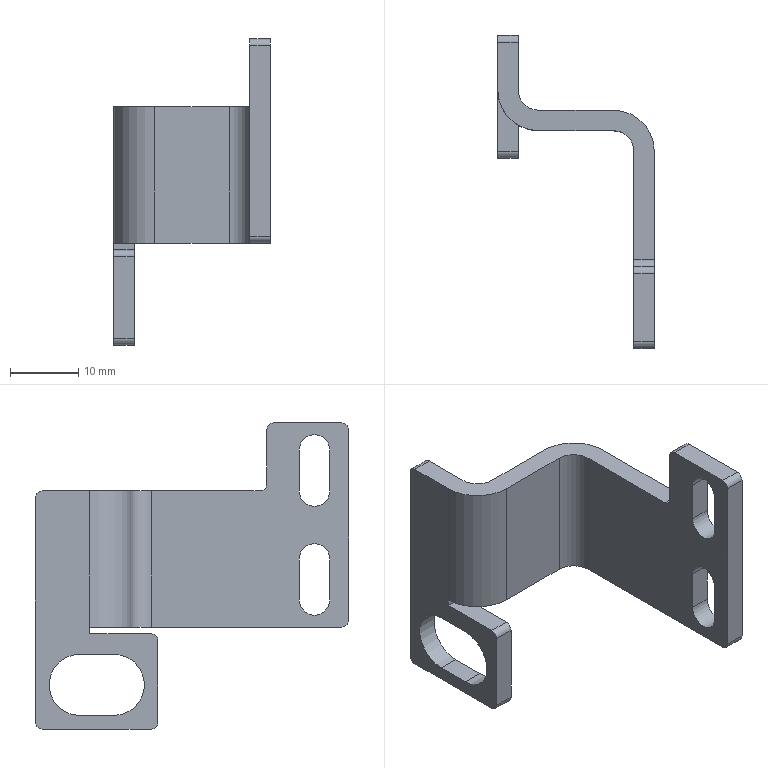Part | NX | features BREP 1 | 1 solid | 43 faces | box 23 x 46 x 45 mm | volume 4281 mm3 | plane 25 | cylinder 18 | commonest cylinder face diameters 2 x8 4.5 x4 6 x2 9 x2 12 x2
STEP:
#1=CARTESIAN_POINT('',(-6.,0.,5.));
#2=VERTEX_POINT('',#1);
#3=CARTESIAN_POINT('',(-17.,0.,5.));
#4=VERTEX_POINT('',#3);
#5=CARTESIAN_POINT('',(-20.,0.,5.));
#6=DIRECTION('',(-1.,0.,0.));
#7=VECTOR('',#6,1000.);
#8=LINE('',#5,#7);
#9=EDGE_CURVE('',#2,#4,#8,.T.);
#10=ORIENTED_EDGE('',*,*,#9,.F.);
#11=CARTESIAN_POINT('',(-6.,0.,-15.));
#12=VERTEX_POINT('',#11);
#13=CARTESIAN_POINT('',(-6.,0.,15.));
#14=DIRECTION('',(0.,0.,-1.));
#15=VECTOR('',#14,1000.);
#16=LINE('',#13,#15);
#17=EDGE_CURVE('',#2,#12,#16,.T.);
#18=ORIENTED_EDGE('',*,*,#17,.T.);
#19=CARTESIAN_POINT('',(-17.,0.,-15.));
#20=VERTEX_POINT('',#19);
#21=CARTESIAN_POINT('',(-20.,0.,-15.));
#22=DIRECTION('',(1.,0.,0.));
#23=VECTOR('',#22,1000.);
#24=LINE('',#21,#23);
#25=EDGE_CURVE('',#20,#12,#24,.T.);
#26=ORIENTED_EDGE('',*,*,#25,.F.);
#27=CARTESIAN_POINT('',(-17.,0.,15.));
#28=DIRECTION('',(0.,0.,-1.));
#29=VECTOR('',#28,1000.);
#30=LINE('',#27,#29);
#31=EDGE_CURVE('',#4,#20,#30,.T.);
#32=ORIENTED_EDGE('',*,*,#31,.F.);
#33=EDGE_LOOP('',(#10,#18,#26,#32));
#34=FACE_BOUND('',#33,.T.);
#35=CARTESIAN_POINT('',(-20.,0.,15.));
#36=DIRECTION('',(0.,1.,0.));
#37=DIRECTION('',(0.,0.,-1.));
#38=AXIS2_PLACEMENT_3D('',#35,#36,#37);
#39=PLANE('',#38);
#40=ADVANCED_FACE('',(#34),#39,.T.);
#41=CARTESIAN_POINT('',(-6.,-3.,5.));
#42=VERTEX_POINT('',#41);
#43=CARTESIAN_POINT('',(-6.,-3.,-15.));
#44=VERTEX_POINT('',#43);
#45=CARTESIAN_POINT('',(-6.,-3.,15.));
#46=DIRECTION('',(0.,0.,-1.));
#47=VECTOR('',#46,1000.);
#48=LINE('',#45,#47);
#49=EDGE_CURVE('',#42,#44,#48,.T.);
#50=ORIENTED_EDGE('',*,*,#49,.F.);
#51=CARTESIAN_POINT('',(-17.,-3.,5.));
#52=VERTEX_POINT('',#51);
#53=CARTESIAN_POINT('',(-20.,-3.,5.));
#54=DIRECTION('',(-1.,0.,0.));
#55=VECTOR('',#54,1000.);
#56=LINE('',#53,#55);
#57=EDGE_CURVE('',#42,#52,#56,.T.);
#58=ORIENTED_EDGE('',*,*,#57,.T.);
#59=CARTESIAN_POINT('',(-17.,-3.,-15.));
#60=VERTEX_POINT('',#59);
#61=CARTESIAN_POINT('',(-17.,-3.,15.));
#62=DIRECTION('',(0.,0.,-1.));
#63=VECTOR('',#62,1000.);
#64=LINE('',#61,#63);
#65=EDGE_CURVE('',#52,#60,#64,.T.);
#66=ORIENTED_EDGE('',*,*,#65,.T.);
#67=CARTESIAN_POINT('',(-20.,-3.,-15.));
#68=DIRECTION('',(1.,0.,0.));
#69=VECTOR('',#68,1000.);
#70=LINE('',#67,#69);
#71=EDGE_CURVE('',#60,#44,#70,.T.);
#72=ORIENTED_EDGE('',*,*,#71,.T.);
#73=EDGE_LOOP('',(#50,#58,#66,#72));
#74=FACE_BOUND('',#73,.T.);
#75=CARTESIAN_POINT('',(-20.,-3.,15.));
#76=DIRECTION('',(0.,1.,0.));
#77=DIRECTION('',(0.,0.,-1.));
#78=AXIS2_PLACEMENT_3D('',#75,#76,#77);
#79=PLANE('',#78);
#80=ADVANCED_FACE('',(#74),#79,.F.);
#81=CARTESIAN_POINT('',(0.,-24.,15.));
#82=VERTEX_POINT('',#81);
#83=CARTESIAN_POINT('',(0.,-34.,15.));
#84=VERTEX_POINT('',#83);
#85=CARTESIAN_POINT('',(0.,0.,15.));
#86=DIRECTION('',(0.,-1.,0.));
#87=VECTOR('',#86,1000.);
#88=LINE('',#85,#87);
#89=EDGE_CURVE('',#82,#84,#88,.T.);
#90=ORIENTED_EDGE('',*,*,#89,.F.);
#91=CARTESIAN_POINT('',(-3.,-24.,15.));
#92=VERTEX_POINT('',#91);
#93=CARTESIAN_POINT('',(-3.,-24.,15.));
#94=DIRECTION('',(-1.,0.,0.));
#95=VECTOR('',#94,1000.);
#96=LINE('',#93,#95);
#97=EDGE_CURVE('',#82,#92,#96,.T.);
#98=ORIENTED_EDGE('',*,*,#97,.T.);
#99=CARTESIAN_POINT('',(-3.,-34.,15.));
#100=VERTEX_POINT('',#99);
#101=CARTESIAN_POINT('',(-3.,0.,15.));
#102=DIRECTION('',(0.,-1.,0.));
#103=VECTOR('',#102,1000.);
#104=LINE('',#101,#103);
#105=EDGE_CURVE('',#92,#100,#104,.T.);
#106=ORIENTED_EDGE('',*,*,#105,.T.);
#107=CARTESIAN_POINT('',(-6.,-34.,15.));
#108=DIRECTION('',(1.,0.,0.));
#109=VECTOR('',#108,1000.);
#110=LINE('',#107,#109);
#111=EDGE_CURVE('',#100,#84,#110,.T.);
#112=ORIENTED_EDGE('',*,*,#111,.T.);
#113=EDGE_LOOP('',(#90,#98,#106,#112));
#114=FACE_BOUND('',#113,.T.);
#115=CARTESIAN_POINT('',(-6.,-3.,15.));
#116=DIRECTION('',(0.,0.,1.));
#117=DIRECTION('',(-1.,0.,0.));
#118=AXIS2_PLACEMENT_3D('',#115,#116,#117);
#119=PLANE('',#118);
#120=ADVANCED_FACE('',(#114),#119,.T.);
#121=CARTESIAN_POINT('',(-6.,0.,-15.));
#122=DIRECTION('',(0.,-1.,0.));
#123=VECTOR('',#122,1000.);
#124=LINE('',#121,#123);
#125=EDGE_CURVE('',#12,#44,#124,.T.);
#126=ORIENTED_EDGE('',*,*,#125,.F.);
#127=CARTESIAN_POINT('',(0.,-6.,-15.));
#128=VERTEX_POINT('',#127);
#129=CARTESIAN_POINT('',(-6.,-6.,-15.));
#130=DIRECTION('',(0.,0.,-1.));
#131=DIRECTION('',(1.,0.,0.));
#132=AXIS2_PLACEMENT_3D('',#129,#130,#131);
#133=CIRCLE('',#132,6.);
#134=EDGE_CURVE('',#12,#128,#133,.T.);
#135=ORIENTED_EDGE('',*,*,#134,.T.);
#136=CARTESIAN_POINT('',(-3.,-6.,-15.));
#137=VERTEX_POINT('',#136);
#138=CARTESIAN_POINT('',(-3.,-6.,-15.));
#139=DIRECTION('',(1.,0.,0.));
#140=VECTOR('',#139,1000.);
#141=LINE('',#138,#140);
#142=EDGE_CURVE('',#137,#128,#141,.T.);
#143=ORIENTED_EDGE('',*,*,#142,.F.);
#144=CARTESIAN_POINT('',(-6.,-6.,-15.));
#145=DIRECTION('',(0.,0.,-1.));
#146=DIRECTION('',(1.,0.,0.));
#147=AXIS2_PLACEMENT_3D('',#144,#145,#146);
#148=CIRCLE('',#147,3.);
#149=EDGE_CURVE('',#44,#137,#148,.T.);
#150=ORIENTED_EDGE('',*,*,#149,.F.);
#151=EDGE_LOOP('',(#126,#135,#143,#150));
#152=FACE_BOUND('',#151,.T.);
#153=CARTESIAN_POINT('',(-6.,0.,-15.));
#154=DIRECTION('',(0.,0.,-1.));
#155=DIRECTION('',(1.,0.,0.));
#156=AXIS2_PLACEMENT_3D('',#153,#154,#155);
#157=PLANE('',#156);
#158=ADVANCED_FACE('',(#152),#157,.T.);
#159=CARTESIAN_POINT('',(-17.,0.,-15.));
#160=DIRECTION('',(0.,-1.,0.));
#161=VECTOR('',#160,1000.);
#162=LINE('',#159,#161);
#163=EDGE_CURVE('',#20,#60,#162,.T.);
#164=ORIENTED_EDGE('',*,*,#163,.F.);
#165=ORIENTED_EDGE('',*,*,#25,.T.);
#166=ORIENTED_EDGE('',*,*,#125,.T.);
#167=ORIENTED_EDGE('',*,*,#71,.F.);
#168=EDGE_LOOP('',(#164,#165,#166,#167));
#169=FACE_BOUND('',#168,.T.);
#170=CARTESIAN_POINT('',(-3.,-6.,-15.));
#171=DIRECTION('',(0.,0.,-1.));
#172=DIRECTION('',(1.,0.,0.));
#173=AXIS2_PLACEMENT_3D('',#170,#171,#172);
#174=PLANE('',#173);
#175=ADVANCED_FACE('',(#169),#174,.T.);
#176=CARTESIAN_POINT('',(-3.,-27.75,11.));
#177=VERTEX_POINT('',#176);
#178=CARTESIAN_POINT('',(-3.,-27.75,5.));
#179=VERTEX_POINT('',#178);
#180=CARTESIAN_POINT('',(-3.,-27.75,11.));
#181=DIRECTION('',(0.,0.,-1.));
#182=VECTOR('',#181,1000.);
#183=LINE('',#180,#182);
#184=EDGE_CURVE('',#177,#179,#183,.T.);
#185=ORIENTED_EDGE('',*,*,#184,.F.);
#186=CARTESIAN_POINT('',(-3.,-32.25,11.));
#187=VERTEX_POINT('',#186);
#188=CARTESIAN_POINT('',(-3.,-30.,11.));
#189=DIRECTION('',(-1.,0.,0.));
#190=DIRECTION('',(0.,1.,0.));
#191=AXIS2_PLACEMENT_3D('',#188,#189,#190);
#192=CIRCLE('',#191,2.25);
#193=EDGE_CURVE('',#187,#177,#192,.T.);
#194=ORIENTED_EDGE('',*,*,#193,.F.);
#195=CARTESIAN_POINT('',(-3.,-32.25,5.));
#196=VERTEX_POINT('',#195);
#197=CARTESIAN_POINT('',(-3.,-32.25,11.));
#198=DIRECTION('',(0.,0.,1.));
#199=VECTOR('',#198,1000.);
#200=LINE('',#197,#199);
#201=EDGE_CURVE('',#196,#187,#200,.T.);
#202=ORIENTED_EDGE('',*,*,#201,.F.);
#203=CARTESIAN_POINT('',(-3.,-30.,5.));
#204=DIRECTION('',(-1.,0.,0.));
#205=DIRECTION('',(0.,1.,0.));
#206=AXIS2_PLACEMENT_3D('',#203,#204,#205);
#207=CIRCLE('',#206,2.25);
#208=EDGE_CURVE('',#179,#196,#207,.T.);
#209=ORIENTED_EDGE('',*,*,#208,.F.);
#210=EDGE_LOOP('',(#185,#194,#202,#209));
#211=FACE_BOUND('',#210,.T.);
#212=CARTESIAN_POINT('',(-3.,-27.75,-5.));
#213=VERTEX_POINT('',#212);
#214=CARTESIAN_POINT('',(-3.,-27.75,-11.));
#215=VERTEX_POINT('',#214);
#216=CARTESIAN_POINT('',(-3.,-27.75,-5.));
#217=DIRECTION('',(0.,0.,-1.));
#218=VECTOR('',#217,1000.);
#219=LINE('',#216,#218);
#220=EDGE_CURVE('',#213,#215,#219,.T.);
#221=ORIENTED_EDGE('',*,*,#220,.F.);
#222=CARTESIAN_POINT('',(-3.,-32.25,-5.));
#223=VERTEX_POINT('',#222);
#224=CARTESIAN_POINT('',(-3.,-30.,-5.));
#225=DIRECTION('',(-1.,0.,0.));
#226=DIRECTION('',(0.,1.,0.));
#227=AXIS2_PLACEMENT_3D('',#224,#225,#226);
#228=CIRCLE('',#227,2.25);
#229=EDGE_CURVE('',#223,#213,#228,.T.);
#230=ORIENTED_EDGE('',*,*,#229,.F.);
#231=CARTESIAN_POINT('',(-3.,-32.25,-11.));
#232=VERTEX_POINT('',#231);
#233=CARTESIAN_POINT('',(-3.,-32.25,-5.));
#234=DIRECTION('',(0.,0.,1.));
#235=VECTOR('',#234,1000.);
#236=LINE('',#233,#235);
#237=EDGE_CURVE('',#232,#223,#236,.T.);
#238=ORIENTED_EDGE('',*,*,#237,.F.);
#239=CARTESIAN_POINT('',(-3.,-30.,-11.));
#240=DIRECTION('',(-1.,0.,0.));
#241=DIRECTION('',(0.,1.,0.));
#242=AXIS2_PLACEMENT_3D('',#239,#240,#241);
#243=CIRCLE('',#242,2.25);
#244=EDGE_CURVE('',#215,#232,#243,.T.);
#245=ORIENTED_EDGE('',*,*,#244,.F.);
#246=EDGE_LOOP('',(#221,#230,#238,#245));
#247=FACE_BOUND('',#246,.T.);
#248=CARTESIAN_POINT('',(-3.,-34.,-15.));
#249=VERTEX_POINT('',#248);
#250=CARTESIAN_POINT('',(-3.,0.,-15.));
#251=DIRECTION('',(0.,-1.,0.));
#252=VECTOR('',#251,1000.);
#253=LINE('',#250,#252);
#254=EDGE_CURVE('',#137,#249,#253,.T.);
#255=ORIENTED_EDGE('',*,*,#254,.T.);
#256=CARTESIAN_POINT('',(-3.,-35.,-14.));
#257=VERTEX_POINT('',#256);
#258=CARTESIAN_POINT('',(-3.,-34.,-14.));
#259=DIRECTION('',(-1.,0.,0.));
#260=DIRECTION('',(0.,1.,0.));
#261=AXIS2_PLACEMENT_3D('',#258,#259,#260);
#262=CIRCLE('',#261,1.);
#263=EDGE_CURVE('',#249,#257,#262,.T.);
#264=ORIENTED_EDGE('',*,*,#263,.T.);
#265=CARTESIAN_POINT('',(-3.,-35.,14.));
#266=VERTEX_POINT('',#265);
#267=CARTESIAN_POINT('',(-3.,-35.,15.));
#268=DIRECTION('',(0.,0.,-1.));
#269=VECTOR('',#268,1000.);
#270=LINE('',#267,#269);
#271=EDGE_CURVE('',#266,#257,#270,.T.);
#272=ORIENTED_EDGE('',*,*,#271,.F.);
#273=CARTESIAN_POINT('',(-3.,-34.,14.));
#274=DIRECTION('',(-1.,0.,0.));
#275=DIRECTION('',(0.,1.,0.));
#276=AXIS2_PLACEMENT_3D('',#273,#274,#275);
#277=CIRCLE('',#276,1.);
#278=EDGE_CURVE('',#266,#100,#277,.T.);
#279=ORIENTED_EDGE('',*,*,#278,.T.);
#280=ORIENTED_EDGE('',*,*,#105,.F.);
#281=CARTESIAN_POINT('',(-3.,-23.,14.));
#282=VERTEX_POINT('',#281);
#283=CARTESIAN_POINT('',(-3.,-24.,14.));
#284=DIRECTION('',(-1.,0.,0.));
#285=DIRECTION('',(0.,1.,0.));
#286=AXIS2_PLACEMENT_3D('',#283,#284,#285);
#287=CIRCLE('',#286,1.);
#288=EDGE_CURVE('',#92,#282,#287,.T.);
#289=ORIENTED_EDGE('',*,*,#288,.T.);
#290=CARTESIAN_POINT('',(-3.,-23.,6.));
#291=VERTEX_POINT('',#290);
#292=CARTESIAN_POINT('',(-3.,-23.,15.));
#293=DIRECTION('',(0.,0.,-1.));
#294=VECTOR('',#293,1000.);
#295=LINE('',#292,#294);
#296=EDGE_CURVE('',#282,#291,#295,.T.);
#297=ORIENTED_EDGE('',*,*,#296,.T.);
#298=CARTESIAN_POINT('',(-3.,-22.,5.));
#299=VERTEX_POINT('',#298);
#300=CARTESIAN_POINT('',(-3.,-22.,6.));
#301=DIRECTION('',(1.,0.,0.));
#302=DIRECTION('',(0.,1.,0.));
#303=AXIS2_PLACEMENT_3D('',#300,#301,#302);
#304=CIRCLE('',#303,1.);
#305=EDGE_CURVE('',#291,#299,#304,.T.);
#306=ORIENTED_EDGE('',*,*,#305,.T.);
#307=CARTESIAN_POINT('',(-3.,-6.,5.));
#308=VERTEX_POINT('',#307);
#309=CARTESIAN_POINT('',(-3.,0.,5.));
#310=DIRECTION('',(0.,1.,0.));
#311=VECTOR('',#310,1000.);
#312=LINE('',#309,#311);
#313=EDGE_CURVE('',#299,#308,#312,.T.);
#314=ORIENTED_EDGE('',*,*,#313,.T.);
#315=CARTESIAN_POINT('',(-3.,-6.,15.));
#316=DIRECTION('',(0.,0.,-1.));
#317=VECTOR('',#316,1000.);
#318=LINE('',#315,#317);
#319=EDGE_CURVE('',#308,#137,#318,.T.);
#320=ORIENTED_EDGE('',*,*,#319,.T.);
#321=EDGE_LOOP('',(#255,#264,#272,#279,#280,#289,#297,#306,#314,#320));
#322=FACE_BOUND('',#321,.T.);
#323=CARTESIAN_POINT('',(-3.,0.,15.));
#324=DIRECTION('',(1.,0.,0.));
#325=DIRECTION('',(0.,-1.,0.));
#326=AXIS2_PLACEMENT_3D('',#323,#324,#325);
#327=PLANE('',#326);
#328=ADVANCED_FACE('',(#211,#247,#322),#327,.F.);
#329=ORIENTED_EDGE('',*,*,#271,.T.);
#330=CARTESIAN_POINT('',(0.,-35.,-14.));
#331=VERTEX_POINT('',#330);
#332=CARTESIAN_POINT('',(0.,-35.,-14.));
#333=DIRECTION('',(1.,0.,0.));
#334=VECTOR('',#333,1000.);
#335=LINE('',#332,#334);
#336=EDGE_CURVE('',#257,#331,#335,.T.);
#337=ORIENTED_EDGE('',*,*,#336,.T.);
#338=CARTESIAN_POINT('',(0.,-35.,14.));
#339=VERTEX_POINT('',#338);
#340=CARTESIAN_POINT('',(0.,-35.,15.));
#341=DIRECTION('',(0.,0.,-1.));
#342=VECTOR('',#341,1000.);
#343=LINE('',#340,#342);
#344=EDGE_CURVE('',#339,#331,#343,.T.);
#345=ORIENTED_EDGE('',*,*,#344,.F.);
#346=CARTESIAN_POINT('',(0.,-35.,14.));
#347=DIRECTION('',(-1.,0.,0.));
#348=VECTOR('',#347,1000.);
#349=LINE('',#346,#348);
#350=EDGE_CURVE('',#339,#266,#349,.T.);
#351=ORIENTED_EDGE('',*,*,#350,.T.);
#352=EDGE_LOOP('',(#329,#337,#345,#351));
#353=FACE_BOUND('',#352,.T.);
#354=CARTESIAN_POINT('',(0.,-35.,15.));
#355=DIRECTION('',(0.,-1.,0.));
#356=DIRECTION('',(0.,0.,1.));
#357=AXIS2_PLACEMENT_3D('',#354,#355,#356);
#358=PLANE('',#357);
#359=ADVANCED_FACE('',(#353),#358,.T.);
#360=ORIENTED_EDGE('',*,*,#344,.T.);
#361=CARTESIAN_POINT('',(0.,-34.,-15.));
#362=VERTEX_POINT('',#361);
#363=CARTESIAN_POINT('',(0.,-34.,-14.));
#364=DIRECTION('',(1.,0.,0.));
#365=DIRECTION('',(0.,1.,0.));
#366=AXIS2_PLACEMENT_3D('',#363,#364,#365);
#367=CIRCLE('',#366,1.);
#368=EDGE_CURVE('',#331,#362,#367,.T.);
#369=ORIENTED_EDGE('',*,*,#368,.T.);
#370=CARTESIAN_POINT('',(0.,0.,-15.));
#371=DIRECTION('',(0.,-1.,0.));
#372=VECTOR('',#371,1000.);
#373=LINE('',#370,#372);
#374=EDGE_CURVE('',#128,#362,#373,.T.);
#375=ORIENTED_EDGE('',*,*,#374,.F.);
#376=CARTESIAN_POINT('',(0.,-6.,5.));
#377=VERTEX_POINT('',#376);
#378=CARTESIAN_POINT('',(0.,-6.,15.));
#379=DIRECTION('',(0.,0.,-1.));
#380=VECTOR('',#379,1000.);
#381=LINE('',#378,#380);
#382=EDGE_CURVE('',#377,#128,#381,.T.);
#383=ORIENTED_EDGE('',*,*,#382,.F.);
#384=CARTESIAN_POINT('',(0.,-22.,5.));
#385=VERTEX_POINT('',#384);
#386=CARTESIAN_POINT('',(0.,11.,5.));
#387=DIRECTION('',(0.,1.,0.));
#388=VECTOR('',#387,1000.);
#389=LINE('',#386,#388);
#390=EDGE_CURVE('',#385,#377,#389,.T.);
#391=ORIENTED_EDGE('',*,*,#390,.F.);
#392=CARTESIAN_POINT('',(0.,-23.,6.));
#393=VERTEX_POINT('',#392);
#394=CARTESIAN_POINT('',(0.,-22.,6.));
#395=DIRECTION('',(-1.,0.,0.));
#396=DIRECTION('',(0.,1.,0.));
#397=AXIS2_PLACEMENT_3D('',#394,#395,#396);
#398=CIRCLE('',#397,1.);
#399=EDGE_CURVE('',#385,#393,#398,.T.);
#400=ORIENTED_EDGE('',*,*,#399,.T.);
#401=CARTESIAN_POINT('',(0.,-23.,14.));
#402=VERTEX_POINT('',#401);
#403=CARTESIAN_POINT('',(0.,-23.,5.));
#404=DIRECTION('',(0.,0.,-1.));
#405=VECTOR('',#404,1000.);
#406=LINE('',#403,#405);
#407=EDGE_CURVE('',#402,#393,#406,.T.);
#408=ORIENTED_EDGE('',*,*,#407,.F.);
#409=CARTESIAN_POINT('',(0.,-24.,14.));
#410=DIRECTION('',(1.,0.,0.));
#411=DIRECTION('',(0.,1.,0.));
#412=AXIS2_PLACEMENT_3D('',#409,#410,#411);
#413=CIRCLE('',#412,1.);
#414=EDGE_CURVE('',#402,#82,#413,.T.);
#415=ORIENTED_EDGE('',*,*,#414,.T.);
#416=ORIENTED_EDGE('',*,*,#89,.T.);
#417=CARTESIAN_POINT('',(0.,-34.,14.));
#418=DIRECTION('',(1.,0.,0.));
#419=DIRECTION('',(0.,1.,0.));
#420=AXIS2_PLACEMENT_3D('',#417,#418,#419);
#421=CIRCLE('',#420,1.);
#422=EDGE_CURVE('',#84,#339,#421,.T.);
#423=ORIENTED_EDGE('',*,*,#422,.T.);
#424=EDGE_LOOP('',(#360,#369,#375,#383,#391,#400,#408,#415,#416,#423));
#425=FACE_BOUND('',#424,.T.);
#426=CARTESIAN_POINT('',(0.,-27.75,11.));
#427=VERTEX_POINT('',#426);
#428=CARTESIAN_POINT('',(0.,-32.25,11.));
#429=VERTEX_POINT('',#428);
#430=CARTESIAN_POINT('',(0.,-30.,11.));
#431=DIRECTION('',(1.,0.,0.));
#432=DIRECTION('',(0.,1.,0.));
#433=AXIS2_PLACEMENT_3D('',#430,#431,#432);
#434=CIRCLE('',#433,2.25);
#435=EDGE_CURVE('',#427,#429,#434,.T.);
#436=ORIENTED_EDGE('',*,*,#435,.F.);
#437=CARTESIAN_POINT('',(0.,-27.75,5.));
#438=VERTEX_POINT('',#437);
#439=CARTESIAN_POINT('',(0.,-27.75,11.));
#440=DIRECTION('',(0.,0.,1.));
#441=VECTOR('',#440,1000.);
#442=LINE('',#439,#441);
#443=EDGE_CURVE('',#438,#427,#442,.T.);
#444=ORIENTED_EDGE('',*,*,#443,.F.);
#445=CARTESIAN_POINT('',(0.,-32.25,5.));
#446=VERTEX_POINT('',#445);
#447=CARTESIAN_POINT('',(0.,-30.,5.));
#448=DIRECTION('',(1.,0.,0.));
#449=DIRECTION('',(0.,1.,0.));
#450=AXIS2_PLACEMENT_3D('',#447,#448,#449);
#451=CIRCLE('',#450,2.25);
#452=EDGE_CURVE('',#446,#438,#451,.T.);
#453=ORIENTED_EDGE('',*,*,#452,.F.);
#454=CARTESIAN_POINT('',(0.,-32.25,11.));
#455=DIRECTION('',(0.,0.,-1.));
#456=VECTOR('',#455,1000.);
#457=LINE('',#454,#456);
#458=EDGE_CURVE('',#429,#446,#457,.T.);
#459=ORIENTED_EDGE('',*,*,#458,.F.);
#460=EDGE_LOOP('',(#436,#444,#453,#459));
#461=FACE_BOUND('',#460,.T.);
#462=CARTESIAN_POINT('',(0.,-27.75,-5.));
#463=VERTEX_POINT('',#462);
#464=CARTESIAN_POINT('',(0.,-32.25,-5.));
#465=VERTEX_POINT('',#464);
#466=CARTESIAN_POINT('',(0.,-30.,-5.));
#467=DIRECTION('',(1.,0.,0.));
#468=DIRECTION('',(0.,1.,0.));
#469=AXIS2_PLACEMENT_3D('',#466,#467,#468);
#470=CIRCLE('',#469,2.25);
#471=EDGE_CURVE('',#463,#465,#470,.T.);
#472=ORIENTED_EDGE('',*,*,#471,.F.);
#473=CARTESIAN_POINT('',(0.,-27.75,-11.));
#474=VERTEX_POINT('',#473);
#475=CARTESIAN_POINT('',(0.,-27.75,-5.));
#476=DIRECTION('',(0.,0.,1.));
#477=VECTOR('',#476,1000.);
#478=LINE('',#475,#477);
#479=EDGE_CURVE('',#474,#463,#478,.T.);
#480=ORIENTED_EDGE('',*,*,#479,.F.);
#481=CARTESIAN_POINT('',(0.,-32.25,-11.));
#482=VERTEX_POINT('',#481);
#483=CARTESIAN_POINT('',(0.,-30.,-11.));
#484=DIRECTION('',(1.,0.,0.));
#485=DIRECTION('',(0.,1.,0.));
#486=AXIS2_PLACEMENT_3D('',#483,#484,#485);
#487=CIRCLE('',#486,2.25);
#488=EDGE_CURVE('',#482,#474,#487,.T.);
#489=ORIENTED_EDGE('',*,*,#488,.F.);
#490=CARTESIAN_POINT('',(0.,-32.25,-5.));
#491=DIRECTION('',(0.,0.,-1.));
#492=VECTOR('',#491,1000.);
#493=LINE('',#490,#492);
#494=EDGE_CURVE('',#465,#482,#493,.T.);
#495=ORIENTED_EDGE('',*,*,#494,.F.);
#496=EDGE_LOOP('',(#472,#480,#489,#495));
#497=FACE_BOUND('',#496,.T.);
#498=CARTESIAN_POINT('',(0.,0.,15.));
#499=DIRECTION('',(1.,0.,0.));
#500=DIRECTION('',(0.,-1.,0.));
#501=AXIS2_PLACEMENT_3D('',#498,#499,#500);
#502=PLANE('',#501);
#503=ADVANCED_FACE('',(#425,#461,#497),#502,.T.);
#504=CARTESIAN_POINT('',(-6.,-6.,5.));
#505=DIRECTION('',(0.,0.,1.));
#506=DIRECTION('',(0.,1.,0.));
#507=AXIS2_PLACEMENT_3D('',#504,#505,#506);
#508=CIRCLE('',#507,6.);
#509=EDGE_CURVE('',#377,#2,#508,.T.);
#510=ORIENTED_EDGE('',*,*,#509,.F.);
#511=ORIENTED_EDGE('',*,*,#382,.T.);
#512=ORIENTED_EDGE('',*,*,#134,.F.);
#513=ORIENTED_EDGE('',*,*,#17,.F.);
#514=EDGE_LOOP('',(#510,#511,#512,#513));
#515=FACE_BOUND('',#514,.T.);
#516=CARTESIAN_POINT('',(-6.,-6.,15.));
#517=DIRECTION('',(0.,0.,-1.));
#518=DIRECTION('',(1.,0.,0.));
#519=AXIS2_PLACEMENT_3D('',#516,#517,#518);
#520=CYLINDRICAL_SURFACE('',#519,6.);
#521=ADVANCED_FACE('',(#515),#520,.T.);
#522=ORIENTED_EDGE('',*,*,#319,.F.);
#523=CARTESIAN_POINT('',(-6.,-6.,5.));
#524=DIRECTION('',(0.,0.,1.));
#525=DIRECTION('',(0.,1.,0.));
#526=AXIS2_PLACEMENT_3D('',#523,#524,#525);
#527=CIRCLE('',#526,3.);
#528=EDGE_CURVE('',#308,#42,#527,.T.);
#529=ORIENTED_EDGE('',*,*,#528,.T.);
#530=ORIENTED_EDGE('',*,*,#49,.T.);
#531=ORIENTED_EDGE('',*,*,#149,.T.);
#532=EDGE_LOOP('',(#522,#529,#530,#531));
#533=FACE_BOUND('',#532,.T.);
#534=CARTESIAN_POINT('',(-6.,-6.,15.));
#535=DIRECTION('',(0.,0.,-1.));
#536=DIRECTION('',(1.,0.,0.));
#537=AXIS2_PLACEMENT_3D('',#534,#535,#536);
#538=CYLINDRICAL_SURFACE('',#537,3.);
#539=ADVANCED_FACE('',(#533),#538,.F.);
#540=ORIENTED_EDGE('',*,*,#374,.T.);
#541=CARTESIAN_POINT('',(-3.,-34.,-15.));
#542=DIRECTION('',(-1.,0.,0.));
#543=VECTOR('',#542,1000.);
#544=LINE('',#541,#543);
#545=EDGE_CURVE('',#362,#249,#544,.T.);
#546=ORIENTED_EDGE('',*,*,#545,.T.);
#547=ORIENTED_EDGE('',*,*,#254,.F.);
#548=ORIENTED_EDGE('',*,*,#142,.T.);
#549=EDGE_LOOP('',(#540,#546,#547,#548));
#550=FACE_BOUND('',#549,.T.);
#551=CARTESIAN_POINT('',(-6.,-6.,-15.));
#552=DIRECTION('',(0.,0.,1.));
#553=DIRECTION('',(-1.,0.,0.));
#554=AXIS2_PLACEMENT_3D('',#551,#552,#553);
#555=PLANE('',#554);
#556=ADVANCED_FACE('',(#550),#555,.F.);
#557=CARTESIAN_POINT('',(-20.,3.,-15.));
#558=VERTEX_POINT('',#557);
#559=CARTESIAN_POINT('',(-23.,3.,-15.));
#560=VERTEX_POINT('',#559);
#561=CARTESIAN_POINT('',(-20.,3.,-15.));
#562=DIRECTION('',(-1.,0.,0.));
#563=VECTOR('',#562,1000.);
#564=LINE('',#561,#563);
#565=EDGE_CURVE('',#558,#560,#564,.T.);
#566=ORIENTED_EDGE('',*,*,#565,.F.);
#567=CARTESIAN_POINT('',(-17.,3.,-15.));
#568=DIRECTION('',(0.,0.,-1.));
#569=DIRECTION('',(1.,0.,0.));
#570=AXIS2_PLACEMENT_3D('',#567,#568,#569);
#571=CIRCLE('',#570,3.);
#572=EDGE_CURVE('',#20,#558,#571,.T.);
#573=ORIENTED_EDGE('',*,*,#572,.F.);
#574=ORIENTED_EDGE('',*,*,#163,.T.);
#575=CARTESIAN_POINT('',(-17.,3.,-15.));
#576=DIRECTION('',(0.,0.,-1.));
#577=DIRECTION('',(1.,0.,0.));
#578=AXIS2_PLACEMENT_3D('',#575,#576,#577);
#579=CIRCLE('',#578,6.);
#580=EDGE_CURVE('',#60,#560,#579,.T.);
#581=ORIENTED_EDGE('',*,*,#580,.T.);
#582=EDGE_LOOP('',(#566,#573,#574,#581));
#583=FACE_BOUND('',#582,.T.);
#584=CARTESIAN_POINT('',(-17.,3.,-15.));
#585=DIRECTION('',(0.,0.,-1.));
#586=DIRECTION('',(1.,0.,0.));
#587=AXIS2_PLACEMENT_3D('',#584,#585,#586);
#588=PLANE('',#587);
#589=ADVANCED_FACE('',(#583),#588,.T.);
#590=CARTESIAN_POINT('',(-23.,3.,5.));
#591=VERTEX_POINT('',#590);
#592=CARTESIAN_POINT('',(-17.,3.,5.));
#593=DIRECTION('',(0.,0.,1.));
#594=DIRECTION('',(0.,1.,0.));
#595=AXIS2_PLACEMENT_3D('',#592,#593,#594);
#596=CIRCLE('',#595,6.);
#597=EDGE_CURVE('',#591,#52,#596,.T.);
#598=ORIENTED_EDGE('',*,*,#597,.F.);
#599=CARTESIAN_POINT('',(-23.,3.,0.));
#600=DIRECTION('',(0.,0.,-1.));
#601=VECTOR('',#600,1000.);
#602=LINE('',#599,#601);
#603=EDGE_CURVE('',#591,#560,#602,.T.);
#604=ORIENTED_EDGE('',*,*,#603,.T.);
#605=ORIENTED_EDGE('',*,*,#580,.F.);
#606=ORIENTED_EDGE('',*,*,#65,.F.);
#607=EDGE_LOOP('',(#598,#604,#605,#606));
#608=FACE_BOUND('',#607,.T.);
#609=CARTESIAN_POINT('',(-17.,3.,15.));
#610=DIRECTION('',(0.,0.,1.));
#611=DIRECTION('',(1.,0.,0.));
#612=AXIS2_PLACEMENT_3D('',#609,#610,#611);
#613=CYLINDRICAL_SURFACE('',#612,6.);
#614=ADVANCED_FACE('',(#608),#613,.T.);
#615=CARTESIAN_POINT('',(-20.,3.,5.));
#616=VERTEX_POINT('',#615);
#617=CARTESIAN_POINT('',(-20.,3.,-15.));
#618=DIRECTION('',(0.,0.,1.));
#619=VECTOR('',#618,1000.);
#620=LINE('',#617,#619);
#621=EDGE_CURVE('',#558,#616,#620,.T.);
#622=ORIENTED_EDGE('',*,*,#621,.T.);
#623=CARTESIAN_POINT('',(-17.,3.,5.));
#624=DIRECTION('',(0.,0.,1.));
#625=DIRECTION('',(0.,1.,0.));
#626=AXIS2_PLACEMENT_3D('',#623,#624,#625);
#627=CIRCLE('',#626,3.);
#628=EDGE_CURVE('',#616,#4,#627,.T.);
#629=ORIENTED_EDGE('',*,*,#628,.T.);
#630=ORIENTED_EDGE('',*,*,#31,.T.);
#631=ORIENTED_EDGE('',*,*,#572,.T.);
#632=EDGE_LOOP('',(#622,#629,#630,#631));
#633=FACE_BOUND('',#632,.T.);
#634=CARTESIAN_POINT('',(-17.,3.,15.));
#635=DIRECTION('',(0.,0.,1.));
#636=DIRECTION('',(1.,0.,0.));
#637=AXIS2_PLACEMENT_3D('',#634,#635,#636);
#638=CYLINDRICAL_SURFACE('',#637,3.);
#639=ADVANCED_FACE('',(#633),#638,.F.);
#640=CARTESIAN_POINT('',(-23.,4.5,-28.));
#641=VERTEX_POINT('',#640);
#642=CARTESIAN_POINT('',(-23.,-0.5,-28.));
#643=VERTEX_POINT('',#642);
#644=CARTESIAN_POINT('',(-23.,4.5,-28.));
#645=DIRECTION('',(0.,-1.,0.));
#646=VECTOR('',#645,1000.);
#647=LINE('',#644,#646);
#648=EDGE_CURVE('',#641,#643,#647,.T.);
#649=ORIENTED_EDGE('',*,*,#648,.F.);
#650=CARTESIAN_POINT('',(-23.,4.5,-19.));
#651=VERTEX_POINT('',#650);
#652=CARTESIAN_POINT('',(-23.,4.5,-23.5));
#653=DIRECTION('',(-1.,0.,0.));
#654=DIRECTION('',(0.,1.,0.));
#655=AXIS2_PLACEMENT_3D('',#652,#653,#654);
#656=CIRCLE('',#655,4.5);
#657=EDGE_CURVE('',#651,#641,#656,.T.);
#658=ORIENTED_EDGE('',*,*,#657,.F.);
#659=CARTESIAN_POINT('',(-23.,-0.5,-19.));
#660=VERTEX_POINT('',#659);
#661=CARTESIAN_POINT('',(-23.,4.5,-19.));
#662=DIRECTION('',(0.,1.,0.));
#663=VECTOR('',#662,1000.);
#664=LINE('',#661,#663);
#665=EDGE_CURVE('',#660,#651,#664,.T.);
#666=ORIENTED_EDGE('',*,*,#665,.F.);
#667=CARTESIAN_POINT('',(-23.,-0.5,-23.5));
#668=DIRECTION('',(-1.,0.,0.));
#669=DIRECTION('',(0.,1.,0.));
#670=AXIS2_PLACEMENT_3D('',#667,#668,#669);
#671=CIRCLE('',#670,4.5);
#672=EDGE_CURVE('',#643,#660,#671,.T.);
#673=ORIENTED_EDGE('',*,*,#672,.F.);
#674=EDGE_LOOP('',(#649,#658,#666,#673));
#675=FACE_BOUND('',#674,.T.);
#676=CARTESIAN_POINT('',(-23.,11.,4.));
#677=VERTEX_POINT('',#676);
#678=CARTESIAN_POINT('',(-23.,11.,-29.));
#679=VERTEX_POINT('',#678);
#680=CARTESIAN_POINT('',(-23.,11.,-15.));
#681=DIRECTION('',(0.,0.,-1.));
#682=VECTOR('',#681,1000.);
#683=LINE('',#680,#682);
#684=EDGE_CURVE('',#677,#679,#683,.T.);
#685=ORIENTED_EDGE('',*,*,#684,.T.);
#686=CARTESIAN_POINT('',(-23.,10.,-30.));
#687=VERTEX_POINT('',#686);
#688=CARTESIAN_POINT('',(-23.,10.,-29.));
#689=DIRECTION('',(-1.,0.,0.));
#690=DIRECTION('',(0.,1.,0.));
#691=AXIS2_PLACEMENT_3D('',#688,#689,#690);
#692=CIRCLE('',#691,1.);
#693=EDGE_CURVE('',#679,#687,#692,.T.);
#694=ORIENTED_EDGE('',*,*,#693,.T.);
#695=CARTESIAN_POINT('',(-23.,-6.,-30.));
#696=VERTEX_POINT('',#695);
#697=CARTESIAN_POINT('',(-23.,11.,-30.));
#698=DIRECTION('',(0.,-1.,0.));
#699=VECTOR('',#698,1000.);
#700=LINE('',#697,#699);
#701=EDGE_CURVE('',#687,#696,#700,.T.);
#702=ORIENTED_EDGE('',*,*,#701,.T.);
#703=CARTESIAN_POINT('',(-23.,-7.,-29.));
#704=VERTEX_POINT('',#703);
#705=CARTESIAN_POINT('',(-23.,-6.,-29.));
#706=DIRECTION('',(-1.,0.,0.));
#707=DIRECTION('',(0.,1.,0.));
#708=AXIS2_PLACEMENT_3D('',#705,#706,#707);
#709=CIRCLE('',#708,1.);
#710=EDGE_CURVE('',#696,#704,#709,.T.);
#711=ORIENTED_EDGE('',*,*,#710,.T.);
#712=CARTESIAN_POINT('',(-23.,-7.,-17.));
#713=VERTEX_POINT('',#712);
#714=CARTESIAN_POINT('',(-23.,-7.,-30.));
#715=DIRECTION('',(0.,0.,1.));
#716=VECTOR('',#715,1000.);
#717=LINE('',#714,#716);
#718=EDGE_CURVE('',#704,#713,#717,.T.);
#719=ORIENTED_EDGE('',*,*,#718,.T.);
#720=CARTESIAN_POINT('',(-23.,-6.,-16.));
#721=VERTEX_POINT('',#720);
#722=CARTESIAN_POINT('',(-23.,-6.,-17.));
#723=DIRECTION('',(-1.,0.,0.));
#724=DIRECTION('',(0.,1.,0.));
#725=AXIS2_PLACEMENT_3D('',#722,#723,#724);
#726=CIRCLE('',#725,1.);
#727=EDGE_CURVE('',#713,#721,#726,.T.);
#728=ORIENTED_EDGE('',*,*,#727,.T.);
#729=CARTESIAN_POINT('',(-23.,3.,-16.));
#730=VERTEX_POINT('',#729);
#731=CARTESIAN_POINT('',(-23.,-7.,-16.));
#732=DIRECTION('',(0.,1.,0.));
#733=VECTOR('',#732,1000.);
#734=LINE('',#731,#733);
#735=EDGE_CURVE('',#721,#730,#734,.T.);
#736=ORIENTED_EDGE('',*,*,#735,.T.);
#737=CARTESIAN_POINT('',(-23.,3.,-16.));
#738=DIRECTION('',(0.,0.,1.));
#739=VECTOR('',#738,1000.);
#740=LINE('',#737,#739);
#741=EDGE_CURVE('',#730,#560,#740,.T.);
#742=ORIENTED_EDGE('',*,*,#741,.T.);
#743=ORIENTED_EDGE('',*,*,#603,.F.);
#744=CARTESIAN_POINT('',(-23.,10.,5.));
#745=VERTEX_POINT('',#744);
#746=CARTESIAN_POINT('',(-23.,11.,5.));
#747=DIRECTION('',(0.,-1.,0.));
#748=VECTOR('',#747,1000.);
#749=LINE('',#746,#748);
#750=EDGE_CURVE('',#745,#591,#749,.T.);
#751=ORIENTED_EDGE('',*,*,#750,.F.);
#752=CARTESIAN_POINT('',(-23.,10.,4.));
#753=DIRECTION('',(-1.,0.,0.));
#754=DIRECTION('',(0.,1.,0.));
#755=AXIS2_PLACEMENT_3D('',#752,#753,#754);
#756=CIRCLE('',#755,1.);
#757=EDGE_CURVE('',#745,#677,#756,.T.);
#758=ORIENTED_EDGE('',*,*,#757,.T.);
#759=EDGE_LOOP('',(#685,#694,#702,#711,#719,#728,#736,#742,#743,#751,#758));
#760=FACE_BOUND('',#759,.T.);
#761=CARTESIAN_POINT('',(-23.,0.,0.));
#762=DIRECTION('',(1.,0.,0.));
#763=DIRECTION('',(0.,-1.,0.));
#764=AXIS2_PLACEMENT_3D('',#761,#762,#763);
#765=PLANE('',#764);
#766=ADVANCED_FACE('',(#675,#760),#765,.F.);
#767=CARTESIAN_POINT('',(-20.,4.5,-28.));
#768=VERTEX_POINT('',#767);
#769=CARTESIAN_POINT('',(-20.,4.5,-19.));
#770=VERTEX_POINT('',#769);
#771=CARTESIAN_POINT('',(-20.,4.5,-23.5));
#772=DIRECTION('',(1.,0.,0.));
#773=DIRECTION('',(0.,1.,0.));
#774=AXIS2_PLACEMENT_3D('',#771,#772,#773);
#775=CIRCLE('',#774,4.5);
#776=EDGE_CURVE('',#768,#770,#775,.T.);
#777=ORIENTED_EDGE('',*,*,#776,.F.);
#778=CARTESIAN_POINT('',(-20.,-0.5,-28.));
#779=VERTEX_POINT('',#778);
#780=CARTESIAN_POINT('',(-20.,4.5,-28.));
#781=DIRECTION('',(0.,1.,0.));
#782=VECTOR('',#781,1000.);
#783=LINE('',#780,#782);
#784=EDGE_CURVE('',#779,#768,#783,.T.);
#785=ORIENTED_EDGE('',*,*,#784,.F.);
#786=CARTESIAN_POINT('',(-20.,-0.5,-19.));
#787=VERTEX_POINT('',#786);
#788=CARTESIAN_POINT('',(-20.,-0.5,-23.5));
#789=DIRECTION('',(1.,0.,0.));
#790=DIRECTION('',(0.,1.,0.));
#791=AXIS2_PLACEMENT_3D('',#788,#789,#790);
#792=CIRCLE('',#791,4.5);
#793=EDGE_CURVE('',#787,#779,#792,.T.);
#794=ORIENTED_EDGE('',*,*,#793,.F.);
#795=CARTESIAN_POINT('',(-20.,4.5,-19.));
#796=DIRECTION('',(0.,-1.,0.));
#797=VECTOR('',#796,1000.);
#798=LINE('',#795,#797);
#799=EDGE_CURVE('',#770,#787,#798,.T.);
#800=ORIENTED_EDGE('',*,*,#799,.F.);
#801=EDGE_LOOP('',(#777,#785,#794,#800));
#802=FACE_BOUND('',#801,.T.);
#803=CARTESIAN_POINT('',(-20.,10.,-30.));
#804=VERTEX_POINT('',#803);
#805=CARTESIAN_POINT('',(-20.,-6.,-30.));
#806=VERTEX_POINT('',#805);
#807=CARTESIAN_POINT('',(-20.,11.,-30.));
#808=DIRECTION('',(0.,-1.,0.));
#809=VECTOR('',#808,1000.);
#810=LINE('',#807,#809);
#811=EDGE_CURVE('',#804,#806,#810,.T.);
#812=ORIENTED_EDGE('',*,*,#811,.F.);
#813=CARTESIAN_POINT('',(-20.,11.,-29.));
#814=VERTEX_POINT('',#813);
#815=CARTESIAN_POINT('',(-20.,10.,-29.));
#816=DIRECTION('',(1.,0.,0.));
#817=DIRECTION('',(0.,1.,0.));
#818=AXIS2_PLACEMENT_3D('',#815,#816,#817);
#819=CIRCLE('',#818,1.);
#820=EDGE_CURVE('',#804,#814,#819,.T.);
#821=ORIENTED_EDGE('',*,*,#820,.T.);
#822=CARTESIAN_POINT('',(-20.,11.,4.));
#823=VERTEX_POINT('',#822);
#824=CARTESIAN_POINT('',(-20.,11.,-15.));
#825=DIRECTION('',(0.,0.,-1.));
#826=VECTOR('',#825,1000.);
#827=LINE('',#824,#826);
#828=EDGE_CURVE('',#823,#814,#827,.T.);
#829=ORIENTED_EDGE('',*,*,#828,.F.);
#830=CARTESIAN_POINT('',(-20.,10.,5.));
#831=VERTEX_POINT('',#830);
#832=CARTESIAN_POINT('',(-20.,10.,4.));
#833=DIRECTION('',(1.,0.,0.));
#834=DIRECTION('',(0.,1.,0.));
#835=AXIS2_PLACEMENT_3D('',#832,#833,#834);
#836=CIRCLE('',#835,1.);
#837=EDGE_CURVE('',#823,#831,#836,.T.);
#838=ORIENTED_EDGE('',*,*,#837,.T.);
#839=CARTESIAN_POINT('',(-20.,0.,5.));
#840=DIRECTION('',(0.,1.,0.));
#841=VECTOR('',#840,1000.);
#842=LINE('',#839,#841);
#843=EDGE_CURVE('',#616,#831,#842,.T.);
#844=ORIENTED_EDGE('',*,*,#843,.F.);
#845=ORIENTED_EDGE('',*,*,#621,.F.);
#846=CARTESIAN_POINT('',(-20.,3.,-16.));
#847=VERTEX_POINT('',#846);
#848=CARTESIAN_POINT('',(-20.,3.,-16.));
#849=DIRECTION('',(0.,0.,1.));
#850=VECTOR('',#849,1000.);
#851=LINE('',#848,#850);
#852=EDGE_CURVE('',#847,#558,#851,.T.);
#853=ORIENTED_EDGE('',*,*,#852,.F.);
#854=CARTESIAN_POINT('',(-20.,-6.,-16.));
#855=VERTEX_POINT('',#854);
#856=CARTESIAN_POINT('',(-20.,-7.,-16.));
#857=DIRECTION('',(0.,1.,0.));
#858=VECTOR('',#857,1000.);
#859=LINE('',#856,#858);
#860=EDGE_CURVE('',#855,#847,#859,.T.);
#861=ORIENTED_EDGE('',*,*,#860,.F.);
#862=CARTESIAN_POINT('',(-20.,-7.,-17.));
#863=VERTEX_POINT('',#862);
#864=CARTESIAN_POINT('',(-20.,-6.,-17.));
#865=DIRECTION('',(1.,0.,0.));
#866=DIRECTION('',(0.,1.,0.));
#867=AXIS2_PLACEMENT_3D('',#864,#865,#866);
#868=CIRCLE('',#867,1.);
#869=EDGE_CURVE('',#855,#863,#868,.T.);
#870=ORIENTED_EDGE('',*,*,#869,.T.);
#871=CARTESIAN_POINT('',(-20.,-7.,-29.));
#872=VERTEX_POINT('',#871);
#873=CARTESIAN_POINT('',(-20.,-7.,-30.));
#874=DIRECTION('',(0.,0.,1.));
#875=VECTOR('',#874,1000.);
#876=LINE('',#873,#875);
#877=EDGE_CURVE('',#872,#863,#876,.T.);
#878=ORIENTED_EDGE('',*,*,#877,.F.);
#879=CARTESIAN_POINT('',(-20.,-6.,-29.));
#880=DIRECTION('',(1.,0.,0.));
#881=DIRECTION('',(0.,1.,0.));
#882=AXIS2_PLACEMENT_3D('',#879,#880,#881);
#883=CIRCLE('',#882,1.);
#884=EDGE_CURVE('',#872,#806,#883,.T.);
#885=ORIENTED_EDGE('',*,*,#884,.T.);
#886=EDGE_LOOP('',(#812,#821,#829,#838,#844,#845,#853,#861,#870,#878,#885));
#887=FACE_BOUND('',#886,.T.);
#888=CARTESIAN_POINT('',(-20.,0.,0.));
#889=DIRECTION('',(1.,0.,0.));
#890=DIRECTION('',(0.,-1.,0.));
#891=AXIS2_PLACEMENT_3D('',#888,#889,#890);
#892=PLANE('',#891);
#893=ADVANCED_FACE('',(#802,#887),#892,.T.);
#894=ORIENTED_EDGE('',*,*,#828,.T.);
#895=CARTESIAN_POINT('',(-23.,11.,-29.));
#896=DIRECTION('',(-1.,0.,0.));
#897=VECTOR('',#896,1000.);
#898=LINE('',#895,#897);
#899=EDGE_CURVE('',#814,#679,#898,.T.);
#900=ORIENTED_EDGE('',*,*,#899,.T.);
#901=ORIENTED_EDGE('',*,*,#684,.F.);
#902=CARTESIAN_POINT('',(-23.,11.,4.));
#903=DIRECTION('',(1.,0.,0.));
#904=VECTOR('',#903,1000.);
#905=LINE('',#902,#904);
#906=EDGE_CURVE('',#677,#823,#905,.T.);
#907=ORIENTED_EDGE('',*,*,#906,.T.);
#908=EDGE_LOOP('',(#894,#900,#901,#907));
#909=FACE_BOUND('',#908,.T.);
#910=CARTESIAN_POINT('',(-23.,11.,-15.));
#911=DIRECTION('',(0.,-1.,0.));
#912=DIRECTION('',(-1.,0.,0.));
#913=AXIS2_PLACEMENT_3D('',#910,#911,#912);
#914=PLANE('',#913);
#915=ADVANCED_FACE('',(#909),#914,.F.);
#916=ORIENTED_EDGE('',*,*,#701,.F.);
#917=CARTESIAN_POINT('',(-20.,10.,-30.));
#918=DIRECTION('',(1.,0.,0.));
#919=VECTOR('',#918,1000.);
#920=LINE('',#917,#919);
#921=EDGE_CURVE('',#687,#804,#920,.T.);
#922=ORIENTED_EDGE('',*,*,#921,.T.);
#923=ORIENTED_EDGE('',*,*,#811,.T.);
#924=CARTESIAN_POINT('',(3.431,-6.,-30.));
#925=DIRECTION('',(-1.,0.,0.));
#926=VECTOR('',#925,1000.);
#927=LINE('',#924,#926);
#928=EDGE_CURVE('',#806,#696,#927,.T.);
#929=ORIENTED_EDGE('',*,*,#928,.T.);
#930=EDGE_LOOP('',(#916,#922,#923,#929));
#931=FACE_BOUND('',#930,.T.);
#932=CARTESIAN_POINT('',(3.431,11.,-30.));
#933=DIRECTION('',(0.,0.,-1.));
#934=DIRECTION('',(1.,0.,0.));
#935=AXIS2_PLACEMENT_3D('',#932,#933,#934);
#936=PLANE('',#935);
#937=ADVANCED_FACE('',(#931),#936,.T.);
#938=ORIENTED_EDGE('',*,*,#877,.T.);
#939=CARTESIAN_POINT('',(3.431,-7.,-17.));
#940=DIRECTION('',(-1.,0.,0.));
#941=VECTOR('',#940,1000.);
#942=LINE('',#939,#941);
#943=EDGE_CURVE('',#863,#713,#942,.T.);
#944=ORIENTED_EDGE('',*,*,#943,.T.);
#945=ORIENTED_EDGE('',*,*,#718,.F.);
#946=CARTESIAN_POINT('',(3.431,-7.,-29.));
#947=DIRECTION('',(1.,0.,0.));
#948=VECTOR('',#947,1000.);
#949=LINE('',#946,#948);
#950=EDGE_CURVE('',#704,#872,#949,.T.);
#951=ORIENTED_EDGE('',*,*,#950,.T.);
#952=EDGE_LOOP('',(#938,#944,#945,#951));
#953=FACE_BOUND('',#952,.T.);
#954=CARTESIAN_POINT('',(3.431,-7.,-30.));
#955=DIRECTION('',(0.,-1.,0.));
#956=DIRECTION('',(-1.,0.,0.));
#957=AXIS2_PLACEMENT_3D('',#954,#955,#956);
#958=PLANE('',#957);
#959=ADVANCED_FACE('',(#953),#958,.T.);
#960=ORIENTED_EDGE('',*,*,#735,.F.);
#961=CARTESIAN_POINT('',(3.431,-6.,-16.));
#962=DIRECTION('',(1.,0.,0.));
#963=VECTOR('',#962,1000.);
#964=LINE('',#961,#963);
#965=EDGE_CURVE('',#721,#855,#964,.T.);
#966=ORIENTED_EDGE('',*,*,#965,.T.);
#967=ORIENTED_EDGE('',*,*,#860,.T.);
#968=CARTESIAN_POINT('',(3.431,3.,-16.));
#969=DIRECTION('',(-1.,0.,0.));
#970=VECTOR('',#969,1000.);
#971=LINE('',#968,#970);
#972=EDGE_CURVE('',#847,#730,#971,.T.);
#973=ORIENTED_EDGE('',*,*,#972,.T.);
#974=EDGE_LOOP('',(#960,#966,#967,#973));
#975=FACE_BOUND('',#974,.T.);
#976=CARTESIAN_POINT('',(3.431,-7.,-16.));
#977=DIRECTION('',(0.,0.,1.));
#978=DIRECTION('',(-1.,0.,0.));
#979=AXIS2_PLACEMENT_3D('',#976,#977,#978);
#980=PLANE('',#979);
#981=ADVANCED_FACE('',(#975),#980,.T.);
#982=ORIENTED_EDGE('',*,*,#972,.F.);
#983=ORIENTED_EDGE('',*,*,#852,.T.);
#984=ORIENTED_EDGE('',*,*,#565,.T.);
#985=ORIENTED_EDGE('',*,*,#741,.F.);
#986=EDGE_LOOP('',(#982,#983,#984,#985));
#987=FACE_BOUND('',#986,.T.);
#988=CARTESIAN_POINT('',(3.431,3.,-16.));
#989=DIRECTION('',(0.,-1.,0.));
#990=DIRECTION('',(-1.,0.,0.));
#991=AXIS2_PLACEMENT_3D('',#988,#989,#990);
#992=PLANE('',#991);
#993=ADVANCED_FACE('',(#987),#992,.T.);
#994=ORIENTED_EDGE('',*,*,#229,.T.);
#995=CARTESIAN_POINT('',(-14.424,-27.75,-5.));
#996=DIRECTION('',(1.,0.,0.));
#997=VECTOR('',#996,1000.);
#998=LINE('',#995,#997);
#999=EDGE_CURVE('',#213,#463,#998,.T.);
#1000=ORIENTED_EDGE('',*,*,#999,.T.);
#1001=ORIENTED_EDGE('',*,*,#471,.T.);
#1002=CARTESIAN_POINT('',(-14.424,-32.25,-5.));
#1003=DIRECTION('',(1.,0.,0.));
#1004=VECTOR('',#1003,1000.);
#1005=LINE('',#1002,#1004);
#1006=EDGE_CURVE('',#223,#465,#1005,.T.);
#1007=ORIENTED_EDGE('',*,*,#1006,.F.);
#1008=EDGE_LOOP('',(#994,#1000,#1001,#1007));
#1009=FACE_BOUND('',#1008,.T.);
#1010=CARTESIAN_POINT('',(-14.424,-30.,-5.));
#1011=DIRECTION('',(1.,0.,0.));
#1012=DIRECTION('',(0.,-1.,0.));
#1013=AXIS2_PLACEMENT_3D('',#1010,#1011,#1012);
#1014=CYLINDRICAL_SURFACE('',#1013,2.25);
#1015=ADVANCED_FACE('',(#1009),#1014,.F.);
#1016=ORIENTED_EDGE('',*,*,#220,.T.);
#1017=CARTESIAN_POINT('',(-14.424,-27.75,-11.));
#1018=DIRECTION('',(1.,0.,0.));
#1019=VECTOR('',#1018,1000.);
#1020=LINE('',#1017,#1019);
#1021=EDGE_CURVE('',#215,#474,#1020,.T.);
#1022=ORIENTED_EDGE('',*,*,#1021,.T.);
#1023=ORIENTED_EDGE('',*,*,#479,.T.);
#1024=ORIENTED_EDGE('',*,*,#999,.F.);
#1025=EDGE_LOOP('',(#1016,#1022,#1023,#1024));
#1026=FACE_BOUND('',#1025,.T.);
#1027=CARTESIAN_POINT('',(-14.424,-27.75,-5.));
#1028=DIRECTION('',(0.,1.,0.));
#1029=DIRECTION('',(1.,0.,0.));
#1030=AXIS2_PLACEMENT_3D('',#1027,#1028,#1029);
#1031=PLANE('',#1030);
#1032=ADVANCED_FACE('',(#1026),#1031,.F.);
#1033=ORIENTED_EDGE('',*,*,#244,.T.);
#1034=CARTESIAN_POINT('',(-14.424,-32.25,-11.));
#1035=DIRECTION('',(1.,0.,0.));
#1036=VECTOR('',#1035,1000.);
#1037=LINE('',#1034,#1036);
#1038=EDGE_CURVE('',#232,#482,#1037,.T.);
#1039=ORIENTED_EDGE('',*,*,#1038,.T.);
#1040=ORIENTED_EDGE('',*,*,#488,.T.);
#1041=ORIENTED_EDGE('',*,*,#1021,.F.);
#1042=EDGE_LOOP('',(#1033,#1039,#1040,#1041));
#1043=FACE_BOUND('',#1042,.T.);
#1044=CARTESIAN_POINT('',(-14.424,-30.,-11.));
#1045=DIRECTION('',(1.,0.,0.));
#1046=DIRECTION('',(0.,-1.,0.));
#1047=AXIS2_PLACEMENT_3D('',#1044,#1045,#1046);
#1048=CYLINDRICAL_SURFACE('',#1047,2.25);
#1049=ADVANCED_FACE('',(#1043),#1048,.F.);
#1050=ORIENTED_EDGE('',*,*,#237,.T.);
#1051=ORIENTED_EDGE('',*,*,#1006,.T.);
#1052=ORIENTED_EDGE('',*,*,#494,.T.);
#1053=ORIENTED_EDGE('',*,*,#1038,.F.);
#1054=EDGE_LOOP('',(#1050,#1051,#1052,#1053));
#1055=FACE_BOUND('',#1054,.T.);
#1056=CARTESIAN_POINT('',(-14.424,-32.25,-5.));
#1057=DIRECTION('',(0.,-1.,0.));
#1058=DIRECTION('',(-1.,0.,0.));
#1059=AXIS2_PLACEMENT_3D('',#1056,#1057,#1058);
#1060=PLANE('',#1059);
#1061=ADVANCED_FACE('',(#1055),#1060,.F.);
#1062=ORIENTED_EDGE('',*,*,#193,.T.);
#1063=CARTESIAN_POINT('',(-14.424,-27.75,11.));
#1064=DIRECTION('',(1.,0.,0.));
#1065=VECTOR('',#1064,1000.);
#1066=LINE('',#1063,#1065);
#1067=EDGE_CURVE('',#177,#427,#1066,.T.);
#1068=ORIENTED_EDGE('',*,*,#1067,.T.);
#1069=ORIENTED_EDGE('',*,*,#435,.T.);
#1070=CARTESIAN_POINT('',(-14.424,-32.25,11.));
#1071=DIRECTION('',(1.,0.,0.));
#1072=VECTOR('',#1071,1000.);
#1073=LINE('',#1070,#1072);
#1074=EDGE_CURVE('',#187,#429,#1073,.T.);
#1075=ORIENTED_EDGE('',*,*,#1074,.F.);
#1076=EDGE_LOOP('',(#1062,#1068,#1069,#1075));
#1077=FACE_BOUND('',#1076,.T.);
#1078=CARTESIAN_POINT('',(-14.424,-30.,11.));
#1079=DIRECTION('',(1.,0.,0.));
#1080=DIRECTION('',(0.,-1.,0.));
#1081=AXIS2_PLACEMENT_3D('',#1078,#1079,#1080);
#1082=CYLINDRICAL_SURFACE('',#1081,2.25);
#1083=ADVANCED_FACE('',(#1077),#1082,.F.);
#1084=ORIENTED_EDGE('',*,*,#184,.T.);
#1085=CARTESIAN_POINT('',(-14.424,-27.75,5.));
#1086=DIRECTION('',(1.,0.,0.));
#1087=VECTOR('',#1086,1000.);
#1088=LINE('',#1085,#1087);
#1089=EDGE_CURVE('',#179,#438,#1088,.T.);
#1090=ORIENTED_EDGE('',*,*,#1089,.T.);
#1091=ORIENTED_EDGE('',*,*,#443,.T.);
#1092=ORIENTED_EDGE('',*,*,#1067,.F.);
#1093=EDGE_LOOP('',(#1084,#1090,#1091,#1092));
#1094=FACE_BOUND('',#1093,.T.);
#1095=CARTESIAN_POINT('',(-14.424,-27.75,11.));
#1096=DIRECTION('',(0.,1.,0.));
#1097=DIRECTION('',(1.,0.,0.));
#1098=AXIS2_PLACEMENT_3D('',#1095,#1096,#1097);
#1099=PLANE('',#1098);
#1100=ADVANCED_FACE('',(#1094),#1099,.F.);
#1101=ORIENTED_EDGE('',*,*,#208,.T.);
#1102=CARTESIAN_POINT('',(-14.424,-32.25,5.));
#1103=DIRECTION('',(1.,0.,0.));
#1104=VECTOR('',#1103,1000.);
#1105=LINE('',#1102,#1104);
#1106=EDGE_CURVE('',#196,#446,#1105,.T.);
#1107=ORIENTED_EDGE('',*,*,#1106,.T.);
#1108=ORIENTED_EDGE('',*,*,#452,.T.);
#1109=ORIENTED_EDGE('',*,*,#1089,.F.);
#1110=EDGE_LOOP('',(#1101,#1107,#1108,#1109));
#1111=FACE_BOUND('',#1110,.T.);
#1112=CARTESIAN_POINT('',(-14.424,-30.,5.));
#1113=DIRECTION('',(1.,0.,0.));
#1114=DIRECTION('',(0.,-1.,0.));
#1115=AXIS2_PLACEMENT_3D('',#1112,#1113,#1114);
#1116=CYLINDRICAL_SURFACE('',#1115,2.25);
#1117=ADVANCED_FACE('',(#1111),#1116,.F.);
#1118=ORIENTED_EDGE('',*,*,#201,.T.);
#1119=ORIENTED_EDGE('',*,*,#1074,.T.);
#1120=ORIENTED_EDGE('',*,*,#458,.T.);
#1121=ORIENTED_EDGE('',*,*,#1106,.F.);
#1122=EDGE_LOOP('',(#1118,#1119,#1120,#1121));
#1123=FACE_BOUND('',#1122,.T.);
#1124=CARTESIAN_POINT('',(-14.424,-32.25,11.));
#1125=DIRECTION('',(0.,-1.,0.));
#1126=DIRECTION('',(-1.,0.,0.));
#1127=AXIS2_PLACEMENT_3D('',#1124,#1125,#1126);
#1128=PLANE('',#1127);
#1129=ADVANCED_FACE('',(#1123),#1128,.F.);
#1130=ORIENTED_EDGE('',*,*,#407,.T.);
#1131=CARTESIAN_POINT('',(-3.,-23.,6.));
#1132=DIRECTION('',(-1.,0.,0.));
#1133=VECTOR('',#1132,1000.);
#1134=LINE('',#1131,#1133);
#1135=EDGE_CURVE('',#393,#291,#1134,.T.);
#1136=ORIENTED_EDGE('',*,*,#1135,.T.);
#1137=ORIENTED_EDGE('',*,*,#296,.F.);
#1138=CARTESIAN_POINT('',(0.,-23.,14.));
#1139=DIRECTION('',(1.,0.,0.));
#1140=VECTOR('',#1139,1000.);
#1141=LINE('',#1138,#1140);
#1142=EDGE_CURVE('',#282,#402,#1141,.T.);
#1143=ORIENTED_EDGE('',*,*,#1142,.T.);
#1144=EDGE_LOOP('',(#1130,#1136,#1137,#1143));
#1145=FACE_BOUND('',#1144,.T.);
#1146=CARTESIAN_POINT('',(-58.44,-23.,5.));
#1147=DIRECTION('',(0.,-1.,0.));
#1148=DIRECTION('',(0.,0.,1.));
#1149=AXIS2_PLACEMENT_3D('',#1146,#1147,#1148);
#1150=PLANE('',#1149);
#1151=ADVANCED_FACE('',(#1145),#1150,.F.);
#1152=ORIENTED_EDGE('',*,*,#843,.T.);
#1153=CARTESIAN_POINT('',(-58.44,10.,5.));
#1154=DIRECTION('',(-1.,0.,0.));
#1155=VECTOR('',#1154,1000.);
#1156=LINE('',#1153,#1155);
#1157=EDGE_CURVE('',#831,#745,#1156,.T.);
#1158=ORIENTED_EDGE('',*,*,#1157,.T.);
#1159=ORIENTED_EDGE('',*,*,#750,.T.);
#1160=ORIENTED_EDGE('',*,*,#597,.T.);
#1161=ORIENTED_EDGE('',*,*,#57,.F.);
#1162=ORIENTED_EDGE('',*,*,#528,.F.);
#1163=ORIENTED_EDGE('',*,*,#313,.F.);
#1164=CARTESIAN_POINT('',(0.,-22.,5.));
#1165=DIRECTION('',(1.,0.,0.));
#1166=VECTOR('',#1165,1000.);
#1167=LINE('',#1164,#1166);
#1168=EDGE_CURVE('',#299,#385,#1167,.T.);
#1169=ORIENTED_EDGE('',*,*,#1168,.T.);
#1170=ORIENTED_EDGE('',*,*,#390,.T.);
#1171=ORIENTED_EDGE('',*,*,#509,.T.);
#1172=ORIENTED_EDGE('',*,*,#9,.T.);
#1173=ORIENTED_EDGE('',*,*,#628,.F.);
#1174=EDGE_LOOP('',(#1152,#1158,#1159,#1160,#1161,#1162,#1163,#1169,#1170,#1171,#1172,#1173));
#1175=FACE_BOUND('',#1174,.T.);
#1176=CARTESIAN_POINT('',(-58.44,11.,5.));
#1177=DIRECTION('',(0.,0.,-1.));
#1178=DIRECTION('',(0.,-1.,0.));
#1179=AXIS2_PLACEMENT_3D('',#1176,#1177,#1178);
#1180=PLANE('',#1179);
#1181=ADVANCED_FACE('',(#1175),#1180,.F.);
#1182=ORIENTED_EDGE('',*,*,#784,.T.);
#1183=CARTESIAN_POINT('',(-39.643,4.5,-28.));
#1184=DIRECTION('',(1.,0.,0.));
#1185=VECTOR('',#1184,1000.);
#1186=LINE('',#1183,#1185);
#1187=EDGE_CURVE('',#641,#768,#1186,.T.);
#1188=ORIENTED_EDGE('',*,*,#1187,.F.);
#1189=ORIENTED_EDGE('',*,*,#648,.T.);
#1190=CARTESIAN_POINT('',(-39.643,-0.5,-28.));
#1191=DIRECTION('',(1.,0.,0.));
#1192=VECTOR('',#1191,1000.);
#1193=LINE('',#1190,#1192);
#1194=EDGE_CURVE('',#643,#779,#1193,.T.);
#1195=ORIENTED_EDGE('',*,*,#1194,.T.);
#1196=EDGE_LOOP('',(#1182,#1188,#1189,#1195));
#1197=FACE_BOUND('',#1196,.T.);
#1198=CARTESIAN_POINT('',(-39.643,4.5,-28.));
#1199=DIRECTION('',(0.,0.,-1.));
#1200=DIRECTION('',(1.,0.,0.));
#1201=AXIS2_PLACEMENT_3D('',#1198,#1199,#1200);
#1202=PLANE('',#1201);
#1203=ADVANCED_FACE('',(#1197),#1202,.F.);
#1204=ORIENTED_EDGE('',*,*,#799,.T.);
#1205=CARTESIAN_POINT('',(-39.643,-0.5,-19.));
#1206=DIRECTION('',(1.,0.,0.));
#1207=VECTOR('',#1206,1000.);
#1208=LINE('',#1205,#1207);
#1209=EDGE_CURVE('',#660,#787,#1208,.T.);
#1210=ORIENTED_EDGE('',*,*,#1209,.F.);
#1211=ORIENTED_EDGE('',*,*,#665,.T.);
#1212=CARTESIAN_POINT('',(-39.643,4.5,-19.));
#1213=DIRECTION('',(1.,0.,0.));
#1214=VECTOR('',#1213,1000.);
#1215=LINE('',#1212,#1214);
#1216=EDGE_CURVE('',#651,#770,#1215,.T.);
#1217=ORIENTED_EDGE('',*,*,#1216,.T.);
#1218=EDGE_LOOP('',(#1204,#1210,#1211,#1217));
#1219=FACE_BOUND('',#1218,.T.);
#1220=CARTESIAN_POINT('',(-39.643,4.5,-19.));
#1221=DIRECTION('',(0.,0.,1.));
#1222=DIRECTION('',(-1.,0.,0.));
#1223=AXIS2_PLACEMENT_3D('',#1220,#1221,#1222);
#1224=PLANE('',#1223);
#1225=ADVANCED_FACE('',(#1219),#1224,.F.);
#1226=ORIENTED_EDGE('',*,*,#657,.T.);
#1227=ORIENTED_EDGE('',*,*,#1187,.T.);
#1228=ORIENTED_EDGE('',*,*,#776,.T.);
#1229=ORIENTED_EDGE('',*,*,#1216,.F.);
#1230=EDGE_LOOP('',(#1226,#1227,#1228,#1229));
#1231=FACE_BOUND('',#1230,.T.);
#1232=CARTESIAN_POINT('',(-39.643,4.5,-23.5));
#1233=DIRECTION('',(1.,0.,0.));
#1234=DIRECTION('',(0.,-1.,0.));
#1235=AXIS2_PLACEMENT_3D('',#1232,#1233,#1234);
#1236=CYLINDRICAL_SURFACE('',#1235,4.5);
#1237=ADVANCED_FACE('',(#1231),#1236,.F.);
#1238=ORIENTED_EDGE('',*,*,#672,.T.);
#1239=ORIENTED_EDGE('',*,*,#1209,.T.);
#1240=ORIENTED_EDGE('',*,*,#793,.T.);
#1241=ORIENTED_EDGE('',*,*,#1194,.F.);
#1242=EDGE_LOOP('',(#1238,#1239,#1240,#1241));
#1243=FACE_BOUND('',#1242,.T.);
#1244=CARTESIAN_POINT('',(-39.643,-0.5,-23.5));
#1245=DIRECTION('',(1.,0.,0.));
#1246=DIRECTION('',(0.,-1.,0.));
#1247=AXIS2_PLACEMENT_3D('',#1244,#1245,#1246);
#1248=CYLINDRICAL_SURFACE('',#1247,4.5);
#1249=ADVANCED_FACE('',(#1243),#1248,.F.);
#1250=ORIENTED_EDGE('',*,*,#820,.F.);
#1251=ORIENTED_EDGE('',*,*,#921,.F.);
#1252=ORIENTED_EDGE('',*,*,#693,.F.);
#1253=ORIENTED_EDGE('',*,*,#899,.F.);
#1254=EDGE_LOOP('',(#1250,#1251,#1252,#1253));
#1255=FACE_BOUND('',#1254,.T.);
#1256=CARTESIAN_POINT('',(-23.,10.,-29.));
#1257=DIRECTION('',(1.,0.,0.));
#1258=DIRECTION('',(0.,-1.,0.));
#1259=AXIS2_PLACEMENT_3D('',#1256,#1257,#1258);
#1260=CYLINDRICAL_SURFACE('',#1259,1.);
#1261=ADVANCED_FACE('',(#1255),#1260,.T.);
#1262=ORIENTED_EDGE('',*,*,#757,.F.);
#1263=ORIENTED_EDGE('',*,*,#1157,.F.);
#1264=ORIENTED_EDGE('',*,*,#837,.F.);
#1265=ORIENTED_EDGE('',*,*,#906,.F.);
#1266=EDGE_LOOP('',(#1262,#1263,#1264,#1265));
#1267=FACE_BOUND('',#1266,.T.);
#1268=CARTESIAN_POINT('',(-23.,10.,4.));
#1269=DIRECTION('',(1.,0.,0.));
#1270=DIRECTION('',(0.,-1.,0.));
#1271=AXIS2_PLACEMENT_3D('',#1268,#1269,#1270);
#1272=CYLINDRICAL_SURFACE('',#1271,1.);
#1273=ADVANCED_FACE('',(#1267),#1272,.T.);
#1274=ORIENTED_EDGE('',*,*,#368,.F.);
#1275=ORIENTED_EDGE('',*,*,#336,.F.);
#1276=ORIENTED_EDGE('',*,*,#263,.F.);
#1277=ORIENTED_EDGE('',*,*,#545,.F.);
#1278=EDGE_LOOP('',(#1274,#1275,#1276,#1277));
#1279=FACE_BOUND('',#1278,.T.);
#1280=CARTESIAN_POINT('',(-6.,-34.,-14.));
#1281=DIRECTION('',(1.,0.,0.));
#1282=DIRECTION('',(0.,0.,1.));
#1283=AXIS2_PLACEMENT_3D('',#1280,#1281,#1282);
#1284=CYLINDRICAL_SURFACE('',#1283,1.);
#1285=ADVANCED_FACE('',(#1279),#1284,.T.);
#1286=ORIENTED_EDGE('',*,*,#305,.F.);
#1287=ORIENTED_EDGE('',*,*,#1135,.F.);
#1288=ORIENTED_EDGE('',*,*,#399,.F.);
#1289=ORIENTED_EDGE('',*,*,#1168,.F.);
#1290=EDGE_LOOP('',(#1286,#1287,#1288,#1289));
#1291=FACE_BOUND('',#1290,.T.);
#1292=CARTESIAN_POINT('',(-58.44,-22.,6.));
#1293=DIRECTION('',(-1.,0.,0.));
#1294=DIRECTION('',(0.,1.,0.));
#1295=AXIS2_PLACEMENT_3D('',#1292,#1293,#1294);
#1296=CYLINDRICAL_SURFACE('',#1295,1.);
#1297=ADVANCED_FACE('',(#1291),#1296,.F.);
#1298=ORIENTED_EDGE('',*,*,#288,.F.);
#1299=ORIENTED_EDGE('',*,*,#97,.F.);
#1300=ORIENTED_EDGE('',*,*,#414,.F.);
#1301=ORIENTED_EDGE('',*,*,#1142,.F.);
#1302=EDGE_LOOP('',(#1298,#1299,#1300,#1301));
#1303=FACE_BOUND('',#1302,.T.);
#1304=CARTESIAN_POINT('',(-58.44,-24.,14.));
#1305=DIRECTION('',(-1.,0.,0.));
#1306=DIRECTION('',(0.,1.,0.));
#1307=AXIS2_PLACEMENT_3D('',#1304,#1305,#1306);
#1308=CYLINDRICAL_SURFACE('',#1307,1.);
#1309=ADVANCED_FACE('',(#1303),#1308,.T.);
#1310=ORIENTED_EDGE('',*,*,#422,.F.);
#1311=ORIENTED_EDGE('',*,*,#111,.F.);
#1312=ORIENTED_EDGE('',*,*,#278,.F.);
#1313=ORIENTED_EDGE('',*,*,#350,.F.);
#1314=EDGE_LOOP('',(#1310,#1311,#1312,#1313));
#1315=FACE_BOUND('',#1314,.T.);
#1316=CARTESIAN_POINT('',(0.,-34.,14.));
#1317=DIRECTION('',(-1.,0.,0.));
#1318=DIRECTION('',(0.,0.,-1.));
#1319=AXIS2_PLACEMENT_3D('',#1316,#1317,#1318);
#1320=CYLINDRICAL_SURFACE('',#1319,1.);
#1321=ADVANCED_FACE('',(#1315),#1320,.T.);
#1322=ORIENTED_EDGE('',*,*,#869,.F.);
#1323=ORIENTED_EDGE('',*,*,#965,.F.);
#1324=ORIENTED_EDGE('',*,*,#727,.F.);
#1325=ORIENTED_EDGE('',*,*,#943,.F.);
#1326=EDGE_LOOP('',(#1322,#1323,#1324,#1325));
#1327=FACE_BOUND('',#1326,.T.);
#1328=CARTESIAN_POINT('',(3.431,-6.,-17.));
#1329=DIRECTION('',(-1.,0.,0.));
#1330=DIRECTION('',(0.,1.,0.));
#1331=AXIS2_PLACEMENT_3D('',#1328,#1329,#1330);
#1332=CYLINDRICAL_SURFACE('',#1331,1.);
#1333=ADVANCED_FACE('',(#1327),#1332,.T.);
#1334=ORIENTED_EDGE('',*,*,#884,.F.);
#1335=ORIENTED_EDGE('',*,*,#950,.F.);
#1336=ORIENTED_EDGE('',*,*,#710,.F.);
#1337=ORIENTED_EDGE('',*,*,#928,.F.);
#1338=EDGE_LOOP('',(#1334,#1335,#1336,#1337));
#1339=FACE_BOUND('',#1338,.T.);
#1340=CARTESIAN_POINT('',(3.431,-6.,-29.));
#1341=DIRECTION('',(-1.,0.,0.));
#1342=DIRECTION('',(0.,1.,0.));
#1343=AXIS2_PLACEMENT_3D('',#1340,#1341,#1342);
#1344=CYLINDRICAL_SURFACE('',#1343,1.);
#1345=ADVANCED_FACE('',(#1339),#1344,.T.);
#1346=CLOSED_SHELL('',(#40,#80,#120,#158,#175,#328,#359,#503,#521,#539,#556,#589,#614,#639,#766,#893,#915,#937,#959,#981,#993,#1015,#1032,#1049,#1061,#1083,#1100,#1117,#1129,#1151,#1181,#1203,#1225,#1237,#1249,#1261,#1273,#1285,#1297,#1309,#1321,#1333,#1345));
#1347=MANIFOLD_SOLID_BREP('',#1346);
#1348=(LENGTH_UNIT()NAMED_UNIT(*)SI_UNIT(.MILLI.,.METRE.));
#1349=UNCERTAINTY_MEASURE_WITH_UNIT(LENGTH_MEASURE(0.00001),#1348,'','');
#1350=(NAMED_UNIT(*)PLANE_ANGLE_UNIT()SI_UNIT($,.RADIAN.));
#1351=(NAMED_UNIT(*)SI_UNIT($,.STERADIAN.)SOLID_ANGLE_UNIT());
#1352=(GEOMETRIC_REPRESENTATION_CONTEXT(3)GLOBAL_UNCERTAINTY_ASSIGNED_CONTEXT((#1349))GLOBAL_UNIT_ASSIGNED_CONTEXT((#1348,#1350,#1351))REPRESENTATION_CONTEXT('',''));
#1353=ADVANCED_BREP_SHAPE_REPRESENTATION('',(#1347),#1352);